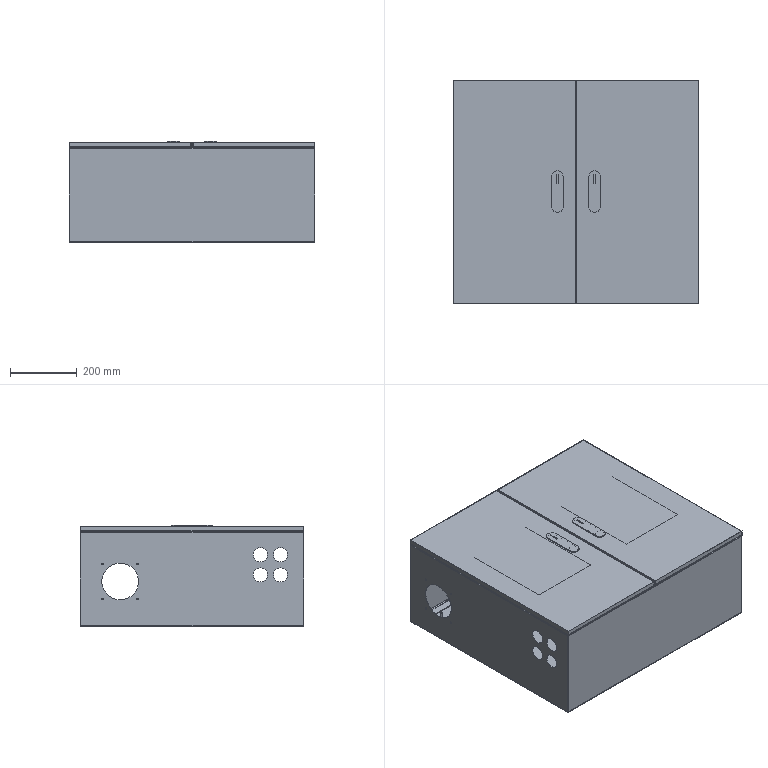Part | SolidWorks | features AEMSimFeature 1, MirrorCompFeat 1, ReferencePattern 1 | 8 solids | 340 faces | box 736 x 670 x 303 mm | volume 3679294 mm3 | plane 180 | cylinder 128 | spline 32 | commonest cylinder face diameters 42 x28 7 x21 5 x16 4 x13 6 x12 1.473 x6